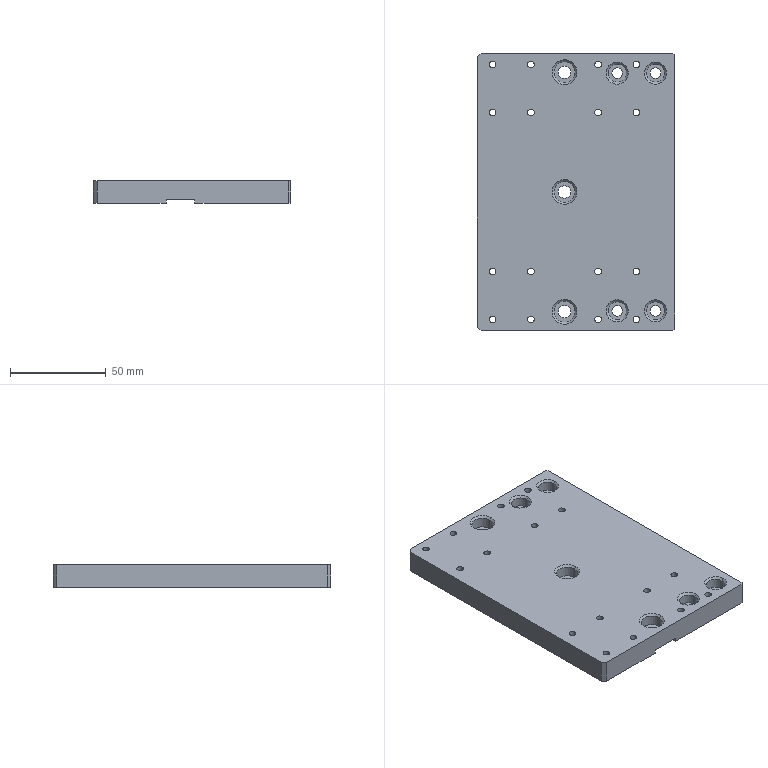Part | STEP file | PN_0007 | 1 solid | 143 faces | box 103 x 145 x 12 mm | volume 167013 mm3 | cylinder 92 | plane 37 | cone 14 | commonest cylinder face diameters 3.5 x32 6 x32 5.5 x8 9.5 x8 6.5 x6 11 x6